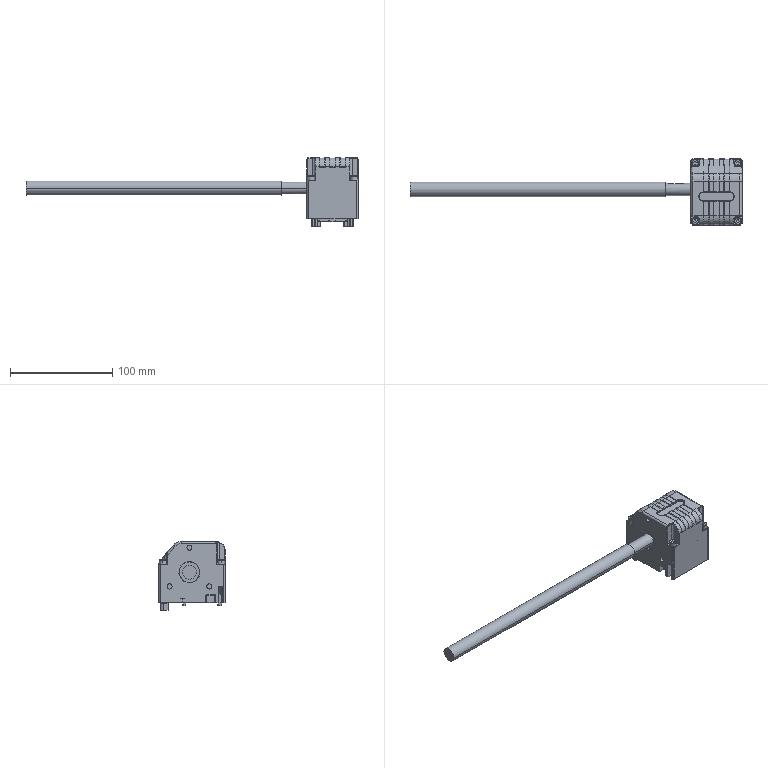Part | STEP file | Copy of K50-right output shaft^K50A-1H20-S(equation-driven)-L | 7 solids | 721 faces | box 325.1 x 65 x 67.5 mm | volume 214031 mm3 | cylinder 297 | plane 210 | spline 188 | cone 26 | commonest cylinder face diameters 1 x85 5 x38 0.4 x24 4 x22 1.6 x18 0.6 x12